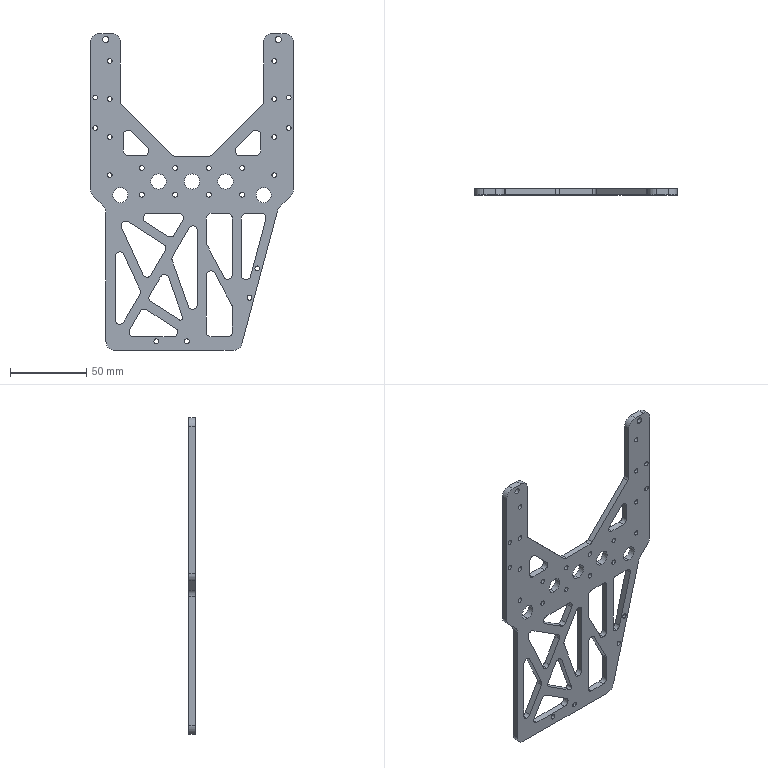Part | SolidWorks | features ICE 8, Fillet 4, Chamfer 1, Extrusion 1 | 1 solid | 169 faces | box 133 x 4 x 208.15 mm | volume 51561 mm3 | cylinder 118 | plane 51 | commonest cylinder face diameters 6 x44 3.2 x32 3.1 x16 10 x10 12 x10 4 x4